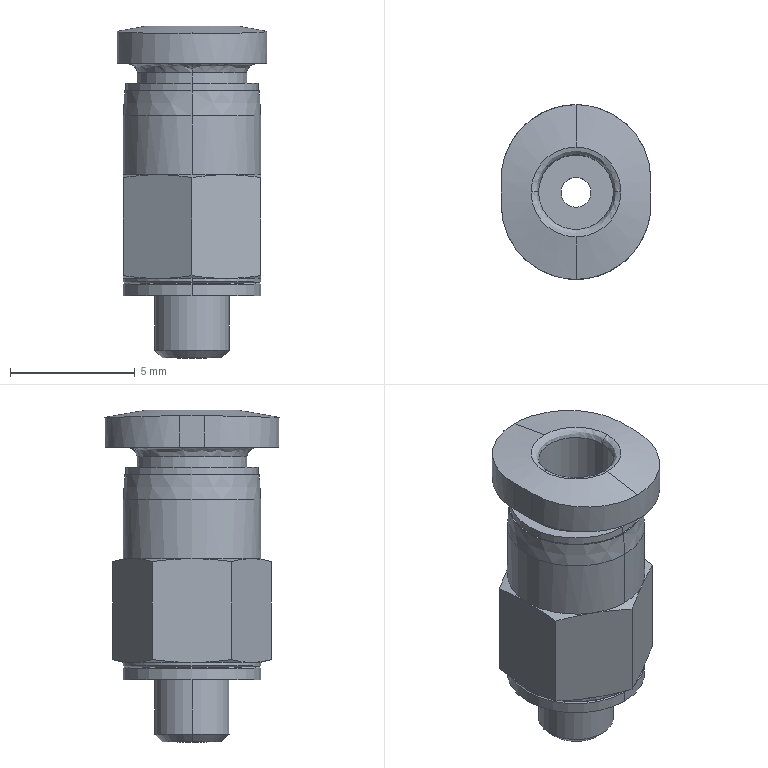Part | SolidWorks | features BaseBody 1 | 1 solid | 60 faces | box 6 x 7 x 13.3 mm | volume 216.387 mm3 | cone 24 | cylinder 18 | plane 14 | spline 4 | commonest cylinder face diameters 5.5 x6 3 x4 1.2 x2 4.4 x2 5.3 x2 6 x2